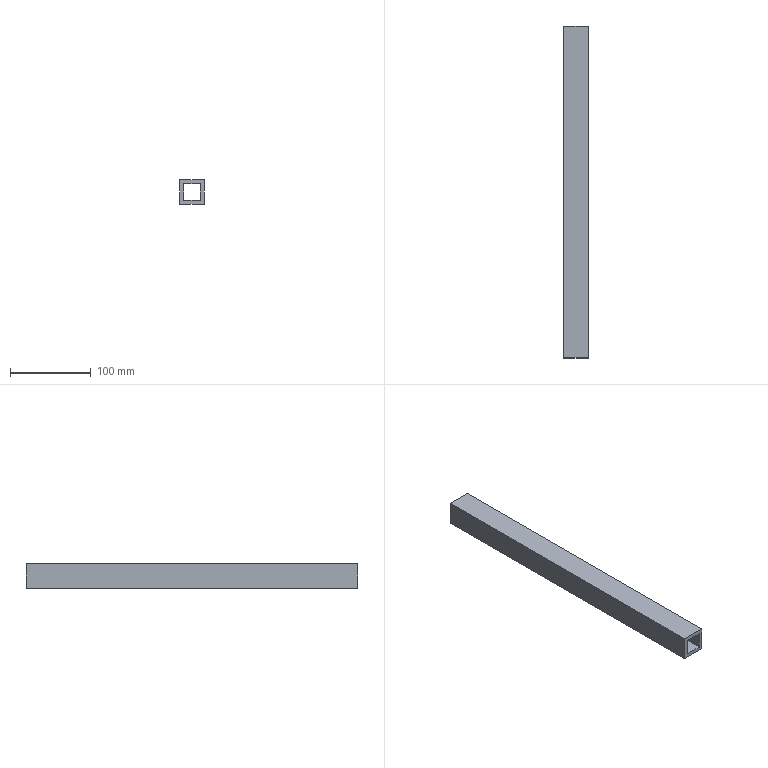Part | NX | features solid 2 | 1 solid | 10 faces | box 30 x 410 x 30 mm | volume 205000 mm3 | plane 10
STEP:
#1=CARTESIAN_POINT('',(-205.,-165.,-50.));
#2=VERTEX_POINT('',#1);
#3=CARTESIAN_POINT('',(-205.,-165.,-80.));
#4=VERTEX_POINT('',#3);
#5=CARTESIAN_POINT('',(-205.,-165.,-50.));
#6=DIRECTION('',(0.,0.,1.));
#7=VECTOR('',#6,1000.);
#8=LINE('',#5,#7);
#9=EDGE_CURVE('',#2,#4,#8,.F.);
#10=ORIENTED_EDGE('',*,*,#9,.F.);
#11=CARTESIAN_POINT('',(-205.,245.,-50.));
#12=VERTEX_POINT('',#11);
#13=CARTESIAN_POINT('',(-205.,20.,-50.));
#14=DIRECTION('',(0.,1.,0.));
#15=VECTOR('',#14,1000.);
#16=LINE('',#13,#15);
#17=EDGE_CURVE('',#2,#12,#16,.T.);
#18=ORIENTED_EDGE('',*,*,#17,.T.);
#19=CARTESIAN_POINT('',(-205.,245.,-80.));
#20=VERTEX_POINT('',#19);
#21=CARTESIAN_POINT('',(-205.,245.,-50.));
#22=DIRECTION('',(0.,0.,1.));
#23=VECTOR('',#22,1000.);
#24=LINE('',#21,#23);
#25=EDGE_CURVE('',#12,#20,#24,.F.);
#26=ORIENTED_EDGE('',*,*,#25,.T.);
#27=CARTESIAN_POINT('',(-205.,20.,-80.));
#28=DIRECTION('',(0.,1.,0.));
#29=VECTOR('',#28,1000.);
#30=LINE('',#27,#29);
#31=EDGE_CURVE('',#4,#20,#30,.T.);
#32=ORIENTED_EDGE('',*,*,#31,.F.);
#33=EDGE_LOOP('',(#10,#18,#26,#32));
#34=FACE_BOUND('',#33,.T.);
#35=CARTESIAN_POINT('',(-205.,20.,-50.));
#36=DIRECTION('',(-1.,0.,0.));
#37=DIRECTION('',(0.,0.,1.));
#38=AXIS2_PLACEMENT_3D('',#35,#36,#37);
#39=PLANE('',#38);
#40=ADVANCED_FACE('',(#34),#39,.T.);
#41=CARTESIAN_POINT('',(-175.,-165.,-50.));
#42=VERTEX_POINT('',#41);
#43=CARTESIAN_POINT('',(-175.,245.,-50.));
#44=VERTEX_POINT('',#43);
#45=CARTESIAN_POINT('',(-175.,20.,-50.));
#46=DIRECTION('',(0.,1.,0.));
#47=VECTOR('',#46,1000.);
#48=LINE('',#45,#47);
#49=EDGE_CURVE('',#42,#44,#48,.T.);
#50=ORIENTED_EDGE('',*,*,#49,.F.);
#51=CARTESIAN_POINT('',(-175.,-165.,-80.));
#52=VERTEX_POINT('',#51);
#53=CARTESIAN_POINT('',(-175.,-165.,-50.));
#54=DIRECTION('',(0.,0.,1.));
#55=VECTOR('',#54,1000.);
#56=LINE('',#53,#55);
#57=EDGE_CURVE('',#42,#52,#56,.F.);
#58=ORIENTED_EDGE('',*,*,#57,.T.);
#59=CARTESIAN_POINT('',(-175.,245.,-80.));
#60=VERTEX_POINT('',#59);
#61=CARTESIAN_POINT('',(-175.,20.,-80.));
#62=DIRECTION('',(0.,1.,0.));
#63=VECTOR('',#62,1000.);
#64=LINE('',#61,#63);
#65=EDGE_CURVE('',#52,#60,#64,.T.);
#66=ORIENTED_EDGE('',*,*,#65,.T.);
#67=CARTESIAN_POINT('',(-175.,245.,-20.));
#68=DIRECTION('',(0.,0.,-1.));
#69=VECTOR('',#68,1000.);
#70=LINE('',#67,#69);
#71=EDGE_CURVE('',#60,#44,#70,.F.);
#72=ORIENTED_EDGE('',*,*,#71,.T.);
#73=EDGE_LOOP('',(#50,#58,#66,#72));
#74=FACE_BOUND('',#73,.T.);
#75=CARTESIAN_POINT('',(-175.,20.,-50.));
#76=DIRECTION('',(-1.,0.,0.));
#77=DIRECTION('',(0.,0.,1.));
#78=AXIS2_PLACEMENT_3D('',#75,#76,#77);
#79=PLANE('',#78);
#80=ADVANCED_FACE('',(#74),#79,.F.);
#81=ORIENTED_EDGE('',*,*,#65,.F.);
#82=CARTESIAN_POINT('',(-205.,-165.,-80.));
#83=DIRECTION('',(1.,0.,0.));
#84=VECTOR('',#83,1000.);
#85=LINE('',#82,#84);
#86=EDGE_CURVE('',#52,#4,#85,.F.);
#87=ORIENTED_EDGE('',*,*,#86,.T.);
#88=ORIENTED_EDGE('',*,*,#31,.T.);
#89=CARTESIAN_POINT('',(-205.,245.,-80.));
#90=DIRECTION('',(1.,0.,0.));
#91=VECTOR('',#90,1000.);
#92=LINE('',#89,#91);
#93=EDGE_CURVE('',#60,#20,#92,.F.);
#94=ORIENTED_EDGE('',*,*,#93,.F.);
#95=EDGE_LOOP('',(#81,#87,#88,#94));
#96=FACE_BOUND('',#95,.T.);
#97=CARTESIAN_POINT('',(-205.,20.,-80.));
#98=DIRECTION('',(0.,0.,1.));
#99=DIRECTION('',(0.,1.,0.));
#100=AXIS2_PLACEMENT_3D('',#97,#98,#99);
#101=PLANE('',#100);
#102=ADVANCED_FACE('',(#96),#101,.F.);
#103=ORIENTED_EDGE('',*,*,#17,.F.);
#104=CARTESIAN_POINT('',(-205.,-165.,-50.));
#105=DIRECTION('',(1.,0.,0.));
#106=VECTOR('',#105,1000.);
#107=LINE('',#104,#106);
#108=EDGE_CURVE('',#2,#42,#107,.T.);
#109=ORIENTED_EDGE('',*,*,#108,.T.);
#110=ORIENTED_EDGE('',*,*,#49,.T.);
#111=CARTESIAN_POINT('',(-205.,245.,-50.));
#112=DIRECTION('',(1.,0.,0.));
#113=VECTOR('',#112,1000.);
#114=LINE('',#111,#113);
#115=EDGE_CURVE('',#12,#44,#114,.T.);
#116=ORIENTED_EDGE('',*,*,#115,.F.);
#117=EDGE_LOOP('',(#103,#109,#110,#116));
#118=FACE_BOUND('',#117,.T.);
#119=CARTESIAN_POINT('',(-205.,20.,-50.));
#120=DIRECTION('',(0.,0.,1.));
#121=DIRECTION('',(0.,1.,0.));
#122=AXIS2_PLACEMENT_3D('',#119,#120,#121);
#123=PLANE('',#122);
#124=ADVANCED_FACE('',(#118),#123,.T.);
#125=CARTESIAN_POINT('',(-200.,-165.,-55.));
#126=VERTEX_POINT('',#125);
#127=CARTESIAN_POINT('',(-200.,245.,-55.));
#128=VERTEX_POINT('',#127);
#129=CARTESIAN_POINT('',(-200.,20.,-55.));
#130=DIRECTION('',(0.,-1.,0.));
#131=VECTOR('',#130,1000.);
#132=LINE('',#129,#131);
#133=EDGE_CURVE('',#126,#128,#132,.F.);
#134=ORIENTED_EDGE('',*,*,#133,.F.);
#135=CARTESIAN_POINT('',(-200.,-165.,-75.));
#136=VERTEX_POINT('',#135);
#137=CARTESIAN_POINT('',(-200.,-165.,-50.));
#138=DIRECTION('',(0.,0.,1.));
#139=VECTOR('',#138,1000.);
#140=LINE('',#137,#139);
#141=EDGE_CURVE('',#126,#136,#140,.F.);
#142=ORIENTED_EDGE('',*,*,#141,.T.);
#143=CARTESIAN_POINT('',(-200.,245.,-75.));
#144=VERTEX_POINT('',#143);
#145=CARTESIAN_POINT('',(-200.,20.,-75.));
#146=DIRECTION('',(0.,1.,0.));
#147=VECTOR('',#146,1000.);
#148=LINE('',#145,#147);
#149=EDGE_CURVE('',#136,#144,#148,.T.);
#150=ORIENTED_EDGE('',*,*,#149,.T.);
#151=CARTESIAN_POINT('',(-200.,245.,-50.));
#152=DIRECTION('',(0.,0.,1.));
#153=VECTOR('',#152,1000.);
#154=LINE('',#151,#153);
#155=EDGE_CURVE('',#128,#144,#154,.F.);
#156=ORIENTED_EDGE('',*,*,#155,.F.);
#157=EDGE_LOOP('',(#134,#142,#150,#156));
#158=FACE_BOUND('',#157,.T.);
#159=CARTESIAN_POINT('',(-200.,20.,-50.));
#160=DIRECTION('',(-1.,0.,0.));
#161=DIRECTION('',(0.,0.,1.));
#162=AXIS2_PLACEMENT_3D('',#159,#160,#161);
#163=PLANE('',#162);
#164=ADVANCED_FACE('',(#158),#163,.F.);
#165=CARTESIAN_POINT('',(-180.,-165.,-55.));
#166=VERTEX_POINT('',#165);
#167=CARTESIAN_POINT('',(-180.,-165.,-75.));
#168=VERTEX_POINT('',#167);
#169=CARTESIAN_POINT('',(-180.,-165.,-50.));
#170=DIRECTION('',(0.,0.,1.));
#171=VECTOR('',#170,1000.);
#172=LINE('',#169,#171);
#173=EDGE_CURVE('',#166,#168,#172,.F.);
#174=ORIENTED_EDGE('',*,*,#173,.F.);
#175=CARTESIAN_POINT('',(-180.,245.,-55.));
#176=VERTEX_POINT('',#175);
#177=CARTESIAN_POINT('',(-180.,20.,-55.));
#178=DIRECTION('',(0.,-1.,0.));
#179=VECTOR('',#178,1000.);
#180=LINE('',#177,#179);
#181=EDGE_CURVE('',#166,#176,#180,.F.);
#182=ORIENTED_EDGE('',*,*,#181,.T.);
#183=CARTESIAN_POINT('',(-180.,245.,-75.));
#184=VERTEX_POINT('',#183);
#185=CARTESIAN_POINT('',(-180.,245.,-20.));
#186=DIRECTION('',(0.,0.,-1.));
#187=VECTOR('',#186,1000.);
#188=LINE('',#185,#187);
#189=EDGE_CURVE('',#184,#176,#188,.F.);
#190=ORIENTED_EDGE('',*,*,#189,.F.);
#191=CARTESIAN_POINT('',(-180.,20.,-75.));
#192=DIRECTION('',(0.,1.,0.));
#193=VECTOR('',#192,1000.);
#194=LINE('',#191,#193);
#195=EDGE_CURVE('',#168,#184,#194,.T.);
#196=ORIENTED_EDGE('',*,*,#195,.F.);
#197=EDGE_LOOP('',(#174,#182,#190,#196));
#198=FACE_BOUND('',#197,.T.);
#199=CARTESIAN_POINT('',(-180.,20.,-50.));
#200=DIRECTION('',(-1.,0.,0.));
#201=DIRECTION('',(0.,0.,1.));
#202=AXIS2_PLACEMENT_3D('',#199,#200,#201);
#203=PLANE('',#202);
#204=ADVANCED_FACE('',(#198),#203,.T.);
#205=CARTESIAN_POINT('',(-205.,-165.,-75.));
#206=DIRECTION('',(1.,0.,0.));
#207=VECTOR('',#206,1000.);
#208=LINE('',#205,#207);
#209=EDGE_CURVE('',#168,#136,#208,.F.);
#210=ORIENTED_EDGE('',*,*,#209,.F.);
#211=ORIENTED_EDGE('',*,*,#195,.T.);
#212=CARTESIAN_POINT('',(-205.,245.,-75.));
#213=DIRECTION('',(1.,0.,0.));
#214=VECTOR('',#213,1000.);
#215=LINE('',#212,#214);
#216=EDGE_CURVE('',#184,#144,#215,.F.);
#217=ORIENTED_EDGE('',*,*,#216,.T.);
#218=ORIENTED_EDGE('',*,*,#149,.F.);
#219=EDGE_LOOP('',(#210,#211,#217,#218));
#220=FACE_BOUND('',#219,.T.);
#221=CARTESIAN_POINT('',(-205.,20.,-75.));
#222=DIRECTION('',(0.,0.,1.));
#223=DIRECTION('',(0.,1.,0.));
#224=AXIS2_PLACEMENT_3D('',#221,#222,#223);
#225=PLANE('',#224);
#226=ADVANCED_FACE('',(#220),#225,.T.);
#227=CARTESIAN_POINT('',(-205.,-165.,-55.));
#228=DIRECTION('',(1.,0.,0.));
#229=VECTOR('',#228,1000.);
#230=LINE('',#227,#229);
#231=EDGE_CURVE('',#126,#166,#230,.T.);
#232=ORIENTED_EDGE('',*,*,#231,.F.);
#233=ORIENTED_EDGE('',*,*,#133,.T.);
#234=CARTESIAN_POINT('',(-205.,245.,-55.));
#235=DIRECTION('',(1.,0.,0.));
#236=VECTOR('',#235,1000.);
#237=LINE('',#234,#236);
#238=EDGE_CURVE('',#128,#176,#237,.T.);
#239=ORIENTED_EDGE('',*,*,#238,.T.);
#240=ORIENTED_EDGE('',*,*,#181,.F.);
#241=EDGE_LOOP('',(#232,#233,#239,#240));
#242=FACE_BOUND('',#241,.T.);
#243=CARTESIAN_POINT('',(-205.,20.,-55.));
#244=DIRECTION('',(0.,0.,1.));
#245=DIRECTION('',(0.,1.,0.));
#246=AXIS2_PLACEMENT_3D('',#243,#244,#245);
#247=PLANE('',#246);
#248=ADVANCED_FACE('',(#242),#247,.F.);
#249=ORIENTED_EDGE('',*,*,#216,.F.);
#250=ORIENTED_EDGE('',*,*,#189,.T.);
#251=ORIENTED_EDGE('',*,*,#238,.F.);
#252=ORIENTED_EDGE('',*,*,#155,.T.);
#253=EDGE_LOOP('',(#249,#250,#251,#252));
#254=FACE_BOUND('',#253,.T.);
#255=ORIENTED_EDGE('',*,*,#71,.F.);
#256=ORIENTED_EDGE('',*,*,#93,.T.);
#257=ORIENTED_EDGE('',*,*,#25,.F.);
#258=ORIENTED_EDGE('',*,*,#115,.T.);
#259=EDGE_LOOP('',(#255,#256,#257,#258));
#260=FACE_BOUND('',#259,.T.);
#261=CARTESIAN_POINT('',(-205.,245.,-20.));
#262=DIRECTION('',(0.,-1.,0.));
#263=DIRECTION('',(0.,0.,-1.));
#264=AXIS2_PLACEMENT_3D('',#261,#262,#263);
#265=PLANE('',#264);
#266=ADVANCED_FACE('',(#254,#260),#265,.F.);
#267=ORIENTED_EDGE('',*,*,#209,.T.);
#268=ORIENTED_EDGE('',*,*,#141,.F.);
#269=ORIENTED_EDGE('',*,*,#231,.T.);
#270=ORIENTED_EDGE('',*,*,#173,.T.);
#271=EDGE_LOOP('',(#267,#268,#269,#270));
#272=FACE_BOUND('',#271,.T.);
#273=ORIENTED_EDGE('',*,*,#57,.F.);
#274=ORIENTED_EDGE('',*,*,#108,.F.);
#275=ORIENTED_EDGE('',*,*,#9,.T.);
#276=ORIENTED_EDGE('',*,*,#86,.F.);
#277=EDGE_LOOP('',(#273,#274,#275,#276));
#278=FACE_BOUND('',#277,.T.);
#279=CARTESIAN_POINT('',(-205.,-165.,-50.));
#280=DIRECTION('',(0.,-1.,0.));
#281=DIRECTION('',(1.,0.,0.));
#282=AXIS2_PLACEMENT_3D('',#279,#280,#281);
#283=PLANE('',#282);
#284=ADVANCED_FACE('',(#272,#278),#283,.T.);
#285=CLOSED_SHELL('',(#40,#80,#102,#124,#164,#204,#226,#248,#266,#284));
#286=MANIFOLD_SOLID_BREP('',#285);
#287=(LENGTH_UNIT()NAMED_UNIT(*)SI_UNIT(.MILLI.,.METRE.));
#288=UNCERTAINTY_MEASURE_WITH_UNIT(LENGTH_MEASURE(0.00001),#287,'','');
#289=(NAMED_UNIT(*)PLANE_ANGLE_UNIT()SI_UNIT($,.RADIAN.));
#290=(NAMED_UNIT(*)SI_UNIT($,.STERADIAN.)SOLID_ANGLE_UNIT());
#291=(GEOMETRIC_REPRESENTATION_CONTEXT(3)GLOBAL_UNCERTAINTY_ASSIGNED_CONTEXT((#288))GLOBAL_UNIT_ASSIGNED_CONTEXT((#287,#289,#290))REPRESENTATION_CONTEXT('',''));
#292=ADVANCED_BREP_SHAPE_REPRESENTATION('',(#286),#291);